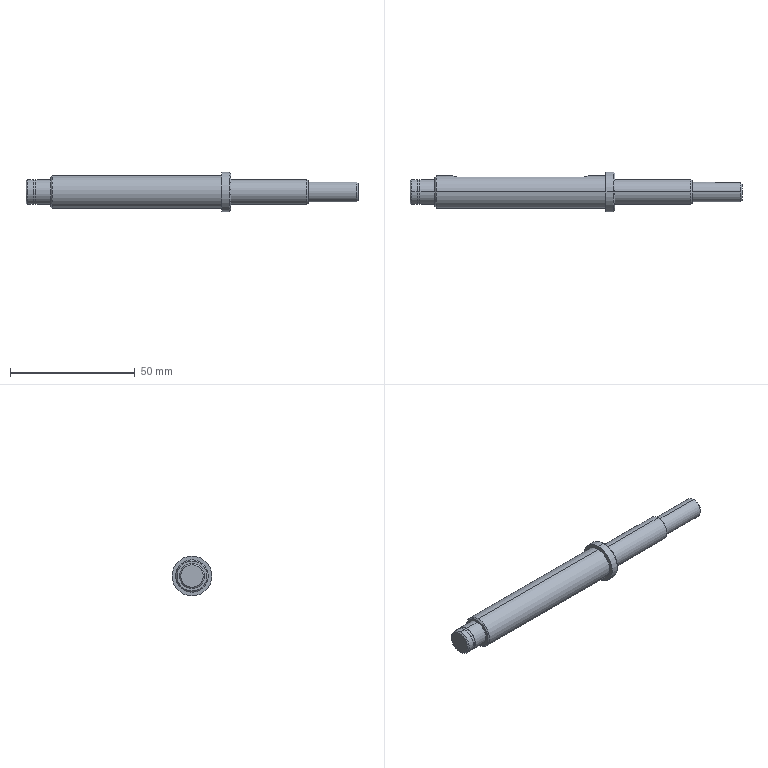Part | SolidWorks | features ICE 2, Chamfer 1, Revolution 1 | 1 solid | 42 faces | box 133 x 16 x 16 mm | volume 13170 mm3 | cylinder 17 | plane 14 | cone 11 | commonest cylinder face diameters 10 x6 5 x2 8 x2 9.6 x2 13 x2 16 x2
STEP:
#1=CARTESIAN_POINT('',(-133.,0.,4.5));
#2=VERTEX_POINT('',#1);
#3=CARTESIAN_POINT('',(-133.,0.,-4.5));
#4=VERTEX_POINT('',#3);
#5=CARTESIAN_POINT('',(-133.,0.,0.));
#6=DIRECTION('',(-1.,0.,0.));
#7=DIRECTION('',(0.,0.,1.));
#8=AXIS2_PLACEMENT_3D('',#5,#6,#7);
#9=CIRCLE('',#8,4.5);
#10=EDGE_CURVE('',#2,#4,#9,.T.);
#11=ORIENTED_EDGE('',*,*,#10,.F.);
#12=CARTESIAN_POINT('',(-132.5,0.,5.));
#13=VERTEX_POINT('',#12);
#14=CARTESIAN_POINT('',(-132.5,0.,5.));
#15=DIRECTION('',(0.7071,0.,0.7071));
#16=VECTOR('',#15,1000.);
#17=LINE('',#14,#16);
#18=EDGE_CURVE('',#2,#13,#17,.T.);
#19=ORIENTED_EDGE('',*,*,#18,.T.);
#20=CARTESIAN_POINT('',(-132.5,0.,-5.));
#21=VERTEX_POINT('',#20);
#22=CARTESIAN_POINT('',(-132.5,0.,0.));
#23=DIRECTION('',(1.,0.,0.));
#24=DIRECTION('',(0.,0.,1.));
#25=AXIS2_PLACEMENT_3D('',#22,#23,#24);
#26=CIRCLE('',#25,5.);
#27=EDGE_CURVE('',#21,#13,#26,.T.);
#28=ORIENTED_EDGE('',*,*,#27,.F.);
#29=CARTESIAN_POINT('',(-132.5,0.,-5.));
#30=DIRECTION('',(0.7071,0.,-0.7071));
#31=VECTOR('',#30,1000.);
#32=LINE('',#29,#31);
#33=EDGE_CURVE('',#4,#21,#32,.T.);
#34=ORIENTED_EDGE('',*,*,#33,.F.);
#35=EDGE_LOOP('',(#11,#19,#28,#34));
#36=FACE_OUTER_BOUND('',#35,.T.);
#37=CARTESIAN_POINT('',(-132.5,0.,0.));
#38=DIRECTION('',(1.,0.,0.));
#39=DIRECTION('',(0.,0.,-1.));
#40=AXIS2_PLACEMENT_3D('',#37,#38,#39);
#41=CONICAL_SURFACE('',#40,5.,0.7854);
#42=ADVANCED_FACE('',(#36),#41,.T.);
#43=CARTESIAN_POINT('',(0.,0.,-3.5));
#44=VERTEX_POINT('',#43);
#45=CARTESIAN_POINT('',(0.,3.162,-1.5));
#46=VERTEX_POINT('',#45);
#47=CARTESIAN_POINT('',(0.,0.,0.));
#48=DIRECTION('',(1.,0.,0.));
#49=DIRECTION('',(0.,0.,-1.));
#50=AXIS2_PLACEMENT_3D('',#47,#48,#49);
#51=CIRCLE('',#50,3.5);
#52=EDGE_CURVE('',#44,#46,#51,.T.);
#53=ORIENTED_EDGE('',*,*,#52,.F.);
#54=CARTESIAN_POINT('',(-0.5,0.,-4.));
#55=VERTEX_POINT('',#54);
#56=CARTESIAN_POINT('',(0.,0.,-3.5));
#57=DIRECTION('',(-0.7071,0.,-0.7071));
#58=VECTOR('',#57,1000.);
#59=LINE('',#56,#58);
#60=EDGE_CURVE('',#44,#55,#59,.T.);
#61=ORIENTED_EDGE('',*,*,#60,.T.);
#62=CARTESIAN_POINT('',(-0.5,3.708,-1.5));
#63=VERTEX_POINT('',#62);
#64=CARTESIAN_POINT('',(-0.5,0.,0.));
#65=DIRECTION('',(-1.,0.,0.));
#66=DIRECTION('',(0.,0.,-1.));
#67=AXIS2_PLACEMENT_3D('',#64,#65,#66);
#68=CIRCLE('',#67,4.);
#69=EDGE_CURVE('',#63,#55,#68,.T.);
#70=ORIENTED_EDGE('',*,*,#69,.F.);
#71=CARTESIAN_POINT('',(0.,3.162,-1.5));
#72=CARTESIAN_POINT('',(-0.1654,3.345,-1.5));
#73=CARTESIAN_POINT('',(-0.3323,3.527,-1.5));
#74=CARTESIAN_POINT('',(-0.5,3.708,-1.5));
#75=B_SPLINE_CURVE_WITH_KNOTS('',3,(#71,#72,#73,#74),.UNSPECIFIED.,.F.,.F.,(4,4),(0.,0.0007402),.UNSPECIFIED.);
#76=EDGE_CURVE('',#46,#63,#75,.T.);
#77=ORIENTED_EDGE('',*,*,#76,.F.);
#78=EDGE_LOOP('',(#53,#61,#70,#77));
#79=FACE_OUTER_BOUND('',#78,.T.);
#80=CARTESIAN_POINT('',(0.,0.,0.));
#81=DIRECTION('',(-1.,0.,0.));
#82=DIRECTION('',(0.,0.,1.));
#83=AXIS2_PLACEMENT_3D('',#80,#81,#82);
#84=CONICAL_SURFACE('',#83,3.5,0.7854);
#85=ADVANCED_FACE('',(#79),#84,.T.);
#86=ORIENTED_EDGE('',*,*,#60,.F.);
#87=CARTESIAN_POINT('',(0.,0.,3.5));
#88=VERTEX_POINT('',#87);
#89=CARTESIAN_POINT('',(0.,0.,0.));
#90=DIRECTION('',(1.,0.,0.));
#91=DIRECTION('',(0.,0.,-1.));
#92=AXIS2_PLACEMENT_3D('',#89,#90,#91);
#93=CIRCLE('',#92,3.5);
#94=EDGE_CURVE('',#88,#44,#93,.T.);
#95=ORIENTED_EDGE('',*,*,#94,.F.);
#96=CARTESIAN_POINT('',(-0.5,0.,4.));
#97=VERTEX_POINT('',#96);
#98=CARTESIAN_POINT('',(0.,0.,3.5));
#99=DIRECTION('',(-0.7071,0.,0.7071));
#100=VECTOR('',#99,1000.);
#101=LINE('',#98,#100);
#102=EDGE_CURVE('',#88,#97,#101,.T.);
#103=ORIENTED_EDGE('',*,*,#102,.T.);
#104=CARTESIAN_POINT('',(-0.5,0.,0.));
#105=DIRECTION('',(-1.,0.,0.));
#106=DIRECTION('',(0.,0.,-1.));
#107=AXIS2_PLACEMENT_3D('',#104,#105,#106);
#108=CIRCLE('',#107,4.);
#109=EDGE_CURVE('',#55,#97,#108,.T.);
#110=ORIENTED_EDGE('',*,*,#109,.F.);
#111=EDGE_LOOP('',(#86,#95,#103,#110));
#112=FACE_OUTER_BOUND('',#111,.T.);
#113=CARTESIAN_POINT('',(0.,0.,0.));
#114=DIRECTION('',(-1.,0.,0.));
#115=DIRECTION('',(0.,0.,1.));
#116=AXIS2_PLACEMENT_3D('',#113,#114,#115);
#117=CONICAL_SURFACE('',#116,3.5,0.7854);
#118=ADVANCED_FACE('',(#112),#117,.T.);
#119=CARTESIAN_POINT('',(-20.,0.,-4.5));
#120=VERTEX_POINT('',#119);
#121=CARTESIAN_POINT('',(-20.,0.,4.5));
#122=VERTEX_POINT('',#121);
#123=CARTESIAN_POINT('',(-20.,0.,0.));
#124=DIRECTION('',(1.,0.,0.));
#125=DIRECTION('',(0.,0.,-1.));
#126=AXIS2_PLACEMENT_3D('',#123,#124,#125);
#127=CIRCLE('',#126,4.5);
#128=EDGE_CURVE('',#120,#122,#127,.T.);
#129=ORIENTED_EDGE('',*,*,#128,.F.);
#130=CARTESIAN_POINT('',(-20.5,0.,-5.));
#131=VERTEX_POINT('',#130);
#132=CARTESIAN_POINT('',(-20.,0.,-4.5));
#133=DIRECTION('',(-0.7071,0.,-0.7071));
#134=VECTOR('',#133,1000.);
#135=LINE('',#132,#134);
#136=EDGE_CURVE('',#120,#131,#135,.T.);
#137=ORIENTED_EDGE('',*,*,#136,.T.);
#138=CARTESIAN_POINT('',(-20.5,0.,5.));
#139=VERTEX_POINT('',#138);
#140=CARTESIAN_POINT('',(-20.5,0.,0.));
#141=DIRECTION('',(-1.,0.,0.));
#142=DIRECTION('',(0.,0.,-1.));
#143=AXIS2_PLACEMENT_3D('',#140,#141,#142);
#144=CIRCLE('',#143,5.);
#145=EDGE_CURVE('',#139,#131,#144,.T.);
#146=ORIENTED_EDGE('',*,*,#145,.F.);
#147=CARTESIAN_POINT('',(-20.,0.,4.5));
#148=DIRECTION('',(-0.7071,0.,0.7071));
#149=VECTOR('',#148,1000.);
#150=LINE('',#147,#149);
#151=EDGE_CURVE('',#122,#139,#150,.T.);
#152=ORIENTED_EDGE('',*,*,#151,.F.);
#153=EDGE_LOOP('',(#129,#137,#146,#152));
#154=FACE_OUTER_BOUND('',#153,.T.);
#155=CARTESIAN_POINT('',(-20.,0.,0.));
#156=DIRECTION('',(-1.,0.,0.));
#157=DIRECTION('',(0.,0.,1.));
#158=AXIS2_PLACEMENT_3D('',#155,#156,#157);
#159=CONICAL_SURFACE('',#158,4.5,0.7854);
#160=ADVANCED_FACE('',(#154),#159,.T.);
#161=CARTESIAN_POINT('',(-123.,0.,6.));
#162=VERTEX_POINT('',#161);
#163=CARTESIAN_POINT('',(-123.,0.,-6.));
#164=VERTEX_POINT('',#163);
#165=CARTESIAN_POINT('',(-123.,0.,0.));
#166=DIRECTION('',(-1.,0.,0.));
#167=DIRECTION('',(0.,0.,1.));
#168=AXIS2_PLACEMENT_3D('',#165,#166,#167);
#169=CIRCLE('',#168,6.);
#170=EDGE_CURVE('',#162,#164,#169,.T.);
#171=ORIENTED_EDGE('',*,*,#170,.F.);
#172=CARTESIAN_POINT('',(-122.5,0.,6.5));
#173=VERTEX_POINT('',#172);
#174=CARTESIAN_POINT('',(-122.5,0.,6.5));
#175=DIRECTION('',(0.7071,0.,0.7071));
#176=VECTOR('',#175,1000.);
#177=LINE('',#174,#176);
#178=EDGE_CURVE('',#162,#173,#177,.T.);
#179=ORIENTED_EDGE('',*,*,#178,.T.);
#180=CARTESIAN_POINT('',(-122.5,0.,-6.5));
#181=VERTEX_POINT('',#180);
#182=CARTESIAN_POINT('',(-122.5,0.,0.));
#183=DIRECTION('',(1.,0.,0.));
#184=DIRECTION('',(0.,0.,1.));
#185=AXIS2_PLACEMENT_3D('',#182,#183,#184);
#186=CIRCLE('',#185,6.5);
#187=EDGE_CURVE('',#181,#173,#186,.T.);
#188=ORIENTED_EDGE('',*,*,#187,.F.);
#189=CARTESIAN_POINT('',(-122.5,0.,-6.5));
#190=DIRECTION('',(0.7071,0.,-0.7071));
#191=VECTOR('',#190,1000.);
#192=LINE('',#189,#191);
#193=EDGE_CURVE('',#164,#181,#192,.T.);
#194=ORIENTED_EDGE('',*,*,#193,.F.);
#195=EDGE_LOOP('',(#171,#179,#188,#194));
#196=FACE_OUTER_BOUND('',#195,.T.);
#197=CARTESIAN_POINT('',(-122.5,0.,0.));
#198=DIRECTION('',(1.,0.,0.));
#199=DIRECTION('',(0.,0.,-1.));
#200=AXIS2_PLACEMENT_3D('',#197,#198,#199);
#201=CONICAL_SURFACE('',#200,6.5,0.7854);
#202=ADVANCED_FACE('',(#196),#201,.T.);
#203=CARTESIAN_POINT('',(-51.,0.,-7.5));
#204=VERTEX_POINT('',#203);
#205=CARTESIAN_POINT('',(-51.,0.,7.5));
#206=VERTEX_POINT('',#205);
#207=CARTESIAN_POINT('',(-51.,0.,0.));
#208=DIRECTION('',(1.,0.,0.));
#209=DIRECTION('',(0.,0.,-1.));
#210=AXIS2_PLACEMENT_3D('',#207,#208,#209);
#211=CIRCLE('',#210,7.5);
#212=EDGE_CURVE('',#204,#206,#211,.T.);
#213=ORIENTED_EDGE('',*,*,#212,.F.);
#214=CARTESIAN_POINT('',(-51.5,0.,-8.));
#215=VERTEX_POINT('',#214);
#216=CARTESIAN_POINT('',(-51.,0.,-7.5));
#217=DIRECTION('',(-0.7071,0.,-0.7071));
#218=VECTOR('',#217,1000.);
#219=LINE('',#216,#218);
#220=EDGE_CURVE('',#204,#215,#219,.T.);
#221=ORIENTED_EDGE('',*,*,#220,.T.);
#222=CARTESIAN_POINT('',(-51.5,0.,8.));
#223=VERTEX_POINT('',#222);
#224=CARTESIAN_POINT('',(-51.5,0.,0.));
#225=DIRECTION('',(-1.,0.,0.));
#226=DIRECTION('',(0.,0.,-1.));
#227=AXIS2_PLACEMENT_3D('',#224,#225,#226);
#228=CIRCLE('',#227,8.);
#229=EDGE_CURVE('',#223,#215,#228,.T.);
#230=ORIENTED_EDGE('',*,*,#229,.F.);
#231=CARTESIAN_POINT('',(-51.,0.,7.5));
#232=DIRECTION('',(-0.7071,0.,0.7071));
#233=VECTOR('',#232,1000.);
#234=LINE('',#231,#233);
#235=EDGE_CURVE('',#206,#223,#234,.T.);
#236=ORIENTED_EDGE('',*,*,#235,.F.);
#237=EDGE_LOOP('',(#213,#221,#230,#236));
#238=FACE_OUTER_BOUND('',#237,.T.);
#239=CARTESIAN_POINT('',(-51.,0.,0.));
#240=DIRECTION('',(-1.,0.,0.));
#241=DIRECTION('',(0.,0.,1.));
#242=AXIS2_PLACEMENT_3D('',#239,#240,#241);
#243=CONICAL_SURFACE('',#242,7.5,0.7854);
#244=ADVANCED_FACE('',(#238),#243,.T.);
#245=CARTESIAN_POINT('',(-20.,0.,-4.));
#246=VERTEX_POINT('',#245);
#247=CARTESIAN_POINT('',(-20.,0.,4.));
#248=VERTEX_POINT('',#247);
#249=CARTESIAN_POINT('',(-20.,0.,0.));
#250=DIRECTION('',(1.,0.,0.));
#251=DIRECTION('',(0.,0.,-1.));
#252=AXIS2_PLACEMENT_3D('',#249,#250,#251);
#253=CIRCLE('',#252,4.);
#254=EDGE_CURVE('',#246,#248,#253,.T.);
#255=ORIENTED_EDGE('',*,*,#254,.T.);
#256=CARTESIAN_POINT('',(0.,0.,4.));
#257=DIRECTION('',(1.,0.,0.));
#258=VECTOR('',#257,1000.);
#259=LINE('',#256,#258);
#260=EDGE_CURVE('',#248,#97,#259,.T.);
#261=ORIENTED_EDGE('',*,*,#260,.T.);
#262=CARTESIAN_POINT('',(-0.5,3.708,1.5));
#263=VERTEX_POINT('',#262);
#264=CARTESIAN_POINT('',(-0.5,0.,0.));
#265=DIRECTION('',(-1.,0.,0.));
#266=DIRECTION('',(0.,0.,-1.));
#267=AXIS2_PLACEMENT_3D('',#264,#265,#266);
#268=CIRCLE('',#267,4.);
#269=EDGE_CURVE('',#97,#263,#268,.T.);
#270=ORIENTED_EDGE('',*,*,#269,.T.);
#271=CARTESIAN_POINT('',(-10.,3.708,1.5));
#272=VERTEX_POINT('',#271);
#273=CARTESIAN_POINT('',(0.,3.708,1.5));
#274=DIRECTION('',(1.,0.,0.));
#275=VECTOR('',#274,1000.);
#276=LINE('',#273,#275);
#277=EDGE_CURVE('',#272,#263,#276,.T.);
#278=ORIENTED_EDGE('',*,*,#277,.F.);
#279=CARTESIAN_POINT('',(-10.,3.708,-1.5));
#280=VERTEX_POINT('',#279);
#281=CARTESIAN_POINT('',(-10.,3.708,-1.5));
#282=CARTESIAN_POINT('',(-10.1,3.708,-1.5));
#283=CARTESIAN_POINT('',(-10.198,3.712,-1.49));
#284=CARTESIAN_POINT('',(-10.391,3.727,-1.451));
#285=CARTESIAN_POINT('',(-10.487,3.739,-1.422));
#286=CARTESIAN_POINT('',(-10.758,3.781,-1.309));
#287=CARTESIAN_POINT('',(-10.923,3.819,-1.198));
#288=CARTESIAN_POINT('',(-11.197,3.894,-0.924));
#289=CARTESIAN_POINT('',(-11.309,3.932,-0.7582));
#290=CARTESIAN_POINT('',(-11.422,3.971,-0.488));
#291=CARTESIAN_POINT('',(-11.451,3.982,-0.3926));
#292=CARTESIAN_POINT('',(-11.49,3.996,-0.1986));
#293=CARTESIAN_POINT('',(-11.5,4.,-0.1006));
#294=CARTESIAN_POINT('',(-11.5,4.,0.09712));
#295=CARTESIAN_POINT('',(-11.49,3.996,0.1975));
#296=CARTESIAN_POINT('',(-11.452,3.982,0.3907));
#297=CARTESIAN_POINT('',(-11.423,3.972,0.4847));
#298=CARTESIAN_POINT('',(-11.309,3.932,0.759));
#299=CARTESIAN_POINT('',(-11.198,3.895,0.9229));
#300=CARTESIAN_POINT('',(-10.992,3.838,1.129));
#301=CARTESIAN_POINT('',(-10.917,3.819,1.191));
#302=CARTESIAN_POINT('',(-10.756,3.783,1.299));
#303=CARTESIAN_POINT('',(-10.668,3.767,1.347));
#304=CARTESIAN_POINT('',(-10.398,3.725,1.459));
#305=CARTESIAN_POINT('',(-10.2,3.708,1.5));
#306=CARTESIAN_POINT('',(-10.,3.708,1.5));
#307=B_SPLINE_CURVE_WITH_KNOTS('',3,(#281,#282,#283,#284,#285,#286,#287,#288,#289,#290,#291,#292,#293,#294,#295,#296,#297,#298,#299,#300,#301,#302,#303,#304,#305,#306),.UNSPECIFIED.,.F.,.F.,(4,2,2,2,2,2,2,2,2,2,2,2,4),(0.,0.0002957,0.0005914,0.001183,0.001774,0.00207,0.002366,0.002661,0.002957,0.003548,0.003844,0.00414,0.004731),.UNSPECIFIED.);
#308=EDGE_CURVE('',#280,#272,#307,.T.);
#309=ORIENTED_EDGE('',*,*,#308,.F.);
#310=CARTESIAN_POINT('',(0.,3.708,-1.5));
#311=DIRECTION('',(-1.,0.,0.));
#312=VECTOR('',#311,1000.);
#313=LINE('',#310,#312);
#314=EDGE_CURVE('',#63,#280,#313,.T.);
#315=ORIENTED_EDGE('',*,*,#314,.F.);
#316=ORIENTED_EDGE('',*,*,#69,.T.);
#317=CARTESIAN_POINT('',(0.,0.,-4.));
#318=DIRECTION('',(1.,0.,0.));
#319=VECTOR('',#318,1000.);
#320=LINE('',#317,#319);
#321=EDGE_CURVE('',#246,#55,#320,.T.);
#322=ORIENTED_EDGE('',*,*,#321,.F.);
#323=EDGE_LOOP('',(#255,#261,#270,#278,#309,#315,#316,#322));
#324=FACE_OUTER_BOUND('',#323,.T.);
#325=CARTESIAN_POINT('',(0.,0.,0.));
#326=DIRECTION('',(1.,0.,0.));
#327=DIRECTION('',(0.,0.,-1.));
#328=AXIS2_PLACEMENT_3D('',#325,#326,#327);
#329=CYLINDRICAL_SURFACE('',#328,4.);
#330=ADVANCED_FACE('',(#324),#329,.T.);
#331=CARTESIAN_POINT('',(-51.,0.,-5.));
#332=VERTEX_POINT('',#331);
#333=CARTESIAN_POINT('',(-51.,0.,5.));
#334=VERTEX_POINT('',#333);
#335=CARTESIAN_POINT('',(-51.,0.,0.));
#336=DIRECTION('',(1.,0.,0.));
#337=DIRECTION('',(0.,0.,-1.));
#338=AXIS2_PLACEMENT_3D('',#335,#336,#337);
#339=CIRCLE('',#338,5.);
#340=EDGE_CURVE('',#332,#334,#339,.T.);
#341=ORIENTED_EDGE('',*,*,#340,.T.);
#342=CARTESIAN_POINT('',(0.,0.,5.));
#343=DIRECTION('',(1.,0.,0.));
#344=VECTOR('',#343,1000.);
#345=LINE('',#342,#344);
#346=EDGE_CURVE('',#334,#139,#345,.T.);
#347=ORIENTED_EDGE('',*,*,#346,.T.);
#348=ORIENTED_EDGE('',*,*,#145,.T.);
#349=CARTESIAN_POINT('',(0.,0.,-5.));
#350=DIRECTION('',(1.,0.,0.));
#351=VECTOR('',#350,1000.);
#352=LINE('',#349,#351);
#353=EDGE_CURVE('',#332,#131,#352,.T.);
#354=ORIENTED_EDGE('',*,*,#353,.F.);
#355=EDGE_LOOP('',(#341,#347,#348,#354));
#356=FACE_OUTER_BOUND('',#355,.T.);
#357=CARTESIAN_POINT('',(0.,0.,0.));
#358=DIRECTION('',(1.,0.,0.));
#359=DIRECTION('',(0.,0.,-1.));
#360=AXIS2_PLACEMENT_3D('',#357,#358,#359);
#361=CYLINDRICAL_SURFACE('',#360,5.);
#362=ADVANCED_FACE('',(#356),#361,.T.);
#363=CARTESIAN_POINT('',(-54.5,0.,-8.));
#364=VERTEX_POINT('',#363);
#365=CARTESIAN_POINT('',(-54.5,0.,8.));
#366=VERTEX_POINT('',#365);
#367=CARTESIAN_POINT('',(-54.5,0.,0.));
#368=DIRECTION('',(1.,0.,0.));
#369=DIRECTION('',(0.,0.,-1.));
#370=AXIS2_PLACEMENT_3D('',#367,#368,#369);
#371=CIRCLE('',#370,8.);
#372=EDGE_CURVE('',#364,#366,#371,.T.);
#373=ORIENTED_EDGE('',*,*,#372,.T.);
#374=CARTESIAN_POINT('',(0.,0.,8.));
#375=DIRECTION('',(1.,0.,0.));
#376=VECTOR('',#375,1000.);
#377=LINE('',#374,#376);
#378=EDGE_CURVE('',#366,#223,#377,.T.);
#379=ORIENTED_EDGE('',*,*,#378,.T.);
#380=ORIENTED_EDGE('',*,*,#229,.T.);
#381=CARTESIAN_POINT('',(0.,0.,-8.));
#382=DIRECTION('',(1.,0.,0.));
#383=VECTOR('',#382,1000.);
#384=LINE('',#381,#383);
#385=EDGE_CURVE('',#364,#215,#384,.T.);
#386=ORIENTED_EDGE('',*,*,#385,.F.);
#387=EDGE_LOOP('',(#373,#379,#380,#386));
#388=FACE_OUTER_BOUND('',#387,.T.);
#389=CARTESIAN_POINT('',(0.,0.,0.));
#390=DIRECTION('',(1.,0.,0.));
#391=DIRECTION('',(0.,0.,-1.));
#392=AXIS2_PLACEMENT_3D('',#389,#390,#391);
#393=CYLINDRICAL_SURFACE('',#392,8.);
#394=ADVANCED_FACE('',(#388),#393,.T.);
#395=CARTESIAN_POINT('',(-63.75,6.,2.5));
#396=VERTEX_POINT('',#395);
#397=CARTESIAN_POINT('',(-63.75,6.,-2.5));
#398=VERTEX_POINT('',#397);
#399=CARTESIAN_POINT('',(-63.75,6.,2.5));
#400=CARTESIAN_POINT('',(-63.583,6.,2.5));
#401=CARTESIAN_POINT('',(-63.419,6.007,2.483));
#402=CARTESIAN_POINT('',(-63.098,6.033,2.419));
#403=CARTESIAN_POINT('',(-62.938,6.053,2.37));
#404=CARTESIAN_POINT('',(-62.637,6.101,2.244));
#405=CARTESIAN_POINT('',(-62.494,6.129,2.168));
#406=CARTESIAN_POINT('',(-62.223,6.19,1.986));
#407=CARTESIAN_POINT('',(-62.097,6.223,1.882));
#408=CARTESIAN_POINT('',(-61.754,6.319,1.54));
#409=CARTESIAN_POINT('',(-61.569,6.383,1.264));
#410=CARTESIAN_POINT('',(-61.381,6.451,0.8138));
#411=CARTESIAN_POINT('',(-61.332,6.469,0.6546));
#412=CARTESIAN_POINT('',(-61.267,6.494,0.3312));
#413=CARTESIAN_POINT('',(-61.25,6.5,0.1679));
#414=CARTESIAN_POINT('',(-61.25,6.5,-0.1619));
#415=CARTESIAN_POINT('',(-61.266,6.494,-0.3292));
#416=CARTESIAN_POINT('',(-61.331,6.469,-0.6513));
#417=CARTESIAN_POINT('',(-61.378,6.451,-0.8081));
#418=CARTESIAN_POINT('',(-61.505,6.406,-1.113));
#419=CARTESIAN_POINT('',(-61.583,6.379,-1.256));
#420=CARTESIAN_POINT('',(-61.763,6.32,-1.526));
#421=CARTESIAN_POINT('',(-61.868,6.287,-1.653));
#422=CARTESIAN_POINT('',(-62.097,6.223,-1.882));
#423=CARTESIAN_POINT('',(-62.221,6.19,-1.985));
#424=CARTESIAN_POINT('',(-62.491,6.129,-2.166));
#425=CARTESIAN_POINT('',(-62.636,6.101,-2.244));
#426=CARTESIAN_POINT('',(-63.086,6.029,-2.432));
#427=CARTESIAN_POINT('',(-63.416,6.,-2.5));
#428=CARTESIAN_POINT('',(-63.75,6.,-2.5));
#429=B_SPLINE_CURVE_WITH_KNOTS('',3,(#399,#400,#401,#402,#403,#404,#405,#406,#407,#408,#409,#410,#411,#412,#413,#414,#415,#416,#417,#418,#419,#420,#421,#422,#423,#424,#425,#426,#427,#428),.UNSPECIFIED.,.F.,.F.,(4,2,2,2,2,2,2,2,2,2,2,2,2,2,4),(0.,0.0004931,0.0009861,0.001479,0.001972,0.002958,0.003452,0.003945,0.004438,0.004931,0.005424,0.005917,0.00641,0.006903,0.007889),.UNSPECIFIED.);
#430=EDGE_CURVE('',#396,#398,#429,.T.);
#431=ORIENTED_EDGE('',*,*,#430,.F.);
#432=CARTESIAN_POINT('',(-113.75,6.,2.5));
#433=VERTEX_POINT('',#432);
#434=CARTESIAN_POINT('',(0.,6.,2.5));
#435=DIRECTION('',(1.,0.,0.));
#436=VECTOR('',#435,1000.);
#437=LINE('',#434,#436);
#438=EDGE_CURVE('',#433,#396,#437,.T.);
#439=ORIENTED_EDGE('',*,*,#438,.F.);
#440=CARTESIAN_POINT('',(-113.75,6.,-2.5));
#441=VERTEX_POINT('',#440);
#442=CARTESIAN_POINT('',(-113.75,6.,-2.5));
#443=CARTESIAN_POINT('',(-113.917,6.,-2.5));
#444=CARTESIAN_POINT('',(-114.081,6.007,-2.483));
#445=CARTESIAN_POINT('',(-114.402,6.033,-2.419));
#446=CARTESIAN_POINT('',(-114.562,6.053,-2.37));
#447=CARTESIAN_POINT('',(-114.863,6.101,-2.244));
#448=CARTESIAN_POINT('',(-115.006,6.129,-2.168));
#449=CARTESIAN_POINT('',(-115.277,6.19,-1.986));
#450=CARTESIAN_POINT('',(-115.403,6.223,-1.882));
#451=CARTESIAN_POINT('',(-115.746,6.319,-1.54));
#452=CARTESIAN_POINT('',(-115.931,6.383,-1.264));
#453=CARTESIAN_POINT('',(-116.119,6.451,-0.8138));
#454=CARTESIAN_POINT('',(-116.168,6.469,-0.6546));
#455=CARTESIAN_POINT('',(-116.233,6.494,-0.3312));
#456=CARTESIAN_POINT('',(-116.25,6.5,-0.1679));
#457=CARTESIAN_POINT('',(-116.25,6.5,0.1619));
#458=CARTESIAN_POINT('',(-116.234,6.494,0.3292));
#459=CARTESIAN_POINT('',(-116.169,6.469,0.6513));
#460=CARTESIAN_POINT('',(-116.122,6.451,0.8081));
#461=CARTESIAN_POINT('',(-115.995,6.406,1.113));
#462=CARTESIAN_POINT('',(-115.917,6.379,1.256));
#463=CARTESIAN_POINT('',(-115.737,6.32,1.526));
#464=CARTESIAN_POINT('',(-115.632,6.287,1.653));
#465=CARTESIAN_POINT('',(-115.403,6.223,1.882));
#466=CARTESIAN_POINT('',(-115.279,6.19,1.985));
#467=CARTESIAN_POINT('',(-115.009,6.129,2.166));
#468=CARTESIAN_POINT('',(-114.864,6.101,2.244));
#469=CARTESIAN_POINT('',(-114.414,6.029,2.432));
#470=CARTESIAN_POINT('',(-114.084,6.,2.5));
#471=CARTESIAN_POINT('',(-113.75,6.,2.5));
#472=B_SPLINE_CURVE_WITH_KNOTS('',3,(#442,#443,#444,#445,#446,#447,#448,#449,#450,#451,#452,#453,#454,#455,#456,#457,#458,#459,#460,#461,#462,#463,#464,#465,#466,#467,#468,#469,#470,#471),.UNSPECIFIED.,.F.,.F.,(4,2,2,2,2,2,2,2,2,2,2,2,2,2,4),(0.,0.0004931,0.0009861,0.001479,0.001972,0.002958,0.003452,0.003945,0.004438,0.004931,0.005424,0.005917,0.00641,0.006903,0.007889),.UNSPECIFIED.);
#473=EDGE_CURVE('',#441,#433,#472,.T.);
#474=ORIENTED_EDGE('',*,*,#473,.F.);
#475=CARTESIAN_POINT('',(0.,6.,-2.5));
#476=DIRECTION('',(-1.,0.,0.));
#477=VECTOR('',#476,1000.);
#478=LINE('',#475,#477);
#479=EDGE_CURVE('',#398,#441,#478,.T.);
#480=ORIENTED_EDGE('',*,*,#479,.F.);
#481=EDGE_LOOP('',(#431,#439,#474,#480));
#482=FACE_BOUND('',#481,.T.);
#483=ORIENTED_EDGE('',*,*,#187,.T.);
#484=CARTESIAN_POINT('',(-54.5,0.,6.5));
#485=VERTEX_POINT('',#484);
#486=CARTESIAN_POINT('',(0.,0.,6.5));
#487=DIRECTION('',(1.,0.,0.));
#488=VECTOR('',#487,1000.);
#489=LINE('',#486,#488);
#490=EDGE_CURVE('',#173,#485,#489,.T.);
#491=ORIENTED_EDGE('',*,*,#490,.T.);
#492=CARTESIAN_POINT('',(-54.5,0.,-6.5));
#493=VERTEX_POINT('',#492);
#494=CARTESIAN_POINT('',(-54.5,0.,0.));
#495=DIRECTION('',(1.,0.,0.));
#496=DIRECTION('',(0.,0.,-1.));
#497=AXIS2_PLACEMENT_3D('',#494,#495,#496);
#498=CIRCLE('',#497,6.5);
#499=EDGE_CURVE('',#493,#485,#498,.T.);
#500=ORIENTED_EDGE('',*,*,#499,.F.);
#501=CARTESIAN_POINT('',(0.,0.,-6.5));
#502=DIRECTION('',(1.,0.,0.));
#503=VECTOR('',#502,1000.);
#504=LINE('',#501,#503);
#505=EDGE_CURVE('',#181,#493,#504,.T.);
#506=ORIENTED_EDGE('',*,*,#505,.F.);
#507=EDGE_LOOP('',(#483,#491,#500,#506));
#508=FACE_OUTER_BOUND('',#507,.T.);
#509=CARTESIAN_POINT('',(0.,0.,0.));
#510=DIRECTION('',(1.,0.,0.));
#511=DIRECTION('',(0.,0.,-1.));
#512=AXIS2_PLACEMENT_3D('',#509,#510,#511);
#513=CYLINDRICAL_SURFACE('',#512,6.5);
#514=ADVANCED_FACE('',(#482,#508),#513,.T.);
#515=CARTESIAN_POINT('',(-129.,0.,-5.));
#516=VERTEX_POINT('',#515);
#517=CARTESIAN_POINT('',(-129.,0.,5.));
#518=VERTEX_POINT('',#517);
#519=CARTESIAN_POINT('',(-129.,0.,0.));
#520=DIRECTION('',(1.,0.,0.));
#521=DIRECTION('',(0.,0.,-1.));
#522=AXIS2_PLACEMENT_3D('',#519,#520,#521);
#523=CIRCLE('',#522,5.);
#524=EDGE_CURVE('',#516,#518,#523,.T.);
#525=ORIENTED_EDGE('',*,*,#524,.T.);
#526=CARTESIAN_POINT('',(-123.,0.,5.));
#527=VERTEX_POINT('',#526);
#528=CARTESIAN_POINT('',(0.,0.,5.));
#529=DIRECTION('',(1.,0.,0.));
#530=VECTOR('',#529,1000.);
#531=LINE('',#528,#530);
#532=EDGE_CURVE('',#518,#527,#531,.T.);
#533=ORIENTED_EDGE('',*,*,#532,.T.);
#534=CARTESIAN_POINT('',(-123.,0.,-5.));
#535=VERTEX_POINT('',#534);
#536=CARTESIAN_POINT('',(-123.,0.,0.));
#537=DIRECTION('',(1.,0.,0.));
#538=DIRECTION('',(0.,0.,-1.));
#539=AXIS2_PLACEMENT_3D('',#536,#537,#538);
#540=CIRCLE('',#539,5.);
#541=EDGE_CURVE('',#535,#527,#540,.T.);
#542=ORIENTED_EDGE('',*,*,#541,.F.);
#543=CARTESIAN_POINT('',(0.,0.,-5.));
#544=DIRECTION('',(1.,0.,0.));
#545=VECTOR('',#544,1000.);
#546=LINE('',#543,#545);
#547=EDGE_CURVE('',#516,#535,#546,.T.);
#548=ORIENTED_EDGE('',*,*,#547,.F.);
#549=EDGE_LOOP('',(#525,#533,#542,#548));
#550=FACE_OUTER_BOUND('',#549,.T.);
#551=CARTESIAN_POINT('',(0.,0.,0.));
#552=DIRECTION('',(1.,0.,0.));
#553=DIRECTION('',(0.,0.,-1.));
#554=AXIS2_PLACEMENT_3D('',#551,#552,#553);
#555=CYLINDRICAL_SURFACE('',#554,5.);
#556=ADVANCED_FACE('',(#550),#555,.T.);
#557=CARTESIAN_POINT('',(-130.1,0.,-4.8));
#558=VERTEX_POINT('',#557);
#559=CARTESIAN_POINT('',(-130.1,0.,4.8));
#560=VERTEX_POINT('',#559);
#561=CARTESIAN_POINT('',(-130.1,0.,0.));
#562=DIRECTION('',(1.,0.,0.));
#563=DIRECTION('',(0.,0.,-1.));
#564=AXIS2_PLACEMENT_3D('',#561,#562,#563);
#565=CIRCLE('',#564,4.8);
#566=EDGE_CURVE('',#558,#560,#565,.T.);
#567=ORIENTED_EDGE('',*,*,#566,.T.);
#568=CARTESIAN_POINT('',(-129.,0.,4.8));
#569=VERTEX_POINT('',#568);
#570=CARTESIAN_POINT('',(0.,0.,4.8));
#571=DIRECTION('',(1.,0.,0.));
#572=VECTOR('',#571,1000.);
#573=LINE('',#570,#572);
#574=EDGE_CURVE('',#560,#569,#573,.T.);
#575=ORIENTED_EDGE('',*,*,#574,.T.);
#576=CARTESIAN_POINT('',(-129.,0.,-4.8));
#577=VERTEX_POINT('',#576);
#578=CARTESIAN_POINT('',(-129.,0.,0.));
#579=DIRECTION('',(1.,0.,0.));
#580=DIRECTION('',(0.,0.,-1.));
#581=AXIS2_PLACEMENT_3D('',#578,#579,#580);
#582=CIRCLE('',#581,4.8);
#583=EDGE_CURVE('',#577,#569,#582,.T.);
#584=ORIENTED_EDGE('',*,*,#583,.F.);
#585=CARTESIAN_POINT('',(0.,0.,-4.8));
#586=DIRECTION('',(1.,0.,0.));
#587=VECTOR('',#586,1000.);
#588=LINE('',#585,#587);
#589=EDGE_CURVE('',#558,#577,#588,.T.);
#590=ORIENTED_EDGE('',*,*,#589,.F.);
#591=EDGE_LOOP('',(#567,#575,#584,#590));
#592=FACE_OUTER_BOUND('',#591,.T.);
#593=CARTESIAN_POINT('',(0.,0.,0.));
#594=DIRECTION('',(1.,0.,0.));
#595=DIRECTION('',(0.,0.,-1.));
#596=AXIS2_PLACEMENT_3D('',#593,#594,#595);
#597=CYLINDRICAL_SURFACE('',#596,4.8);
#598=ADVANCED_FACE('',(#592),#597,.T.);
#599=ORIENTED_EDGE('',*,*,#27,.T.);
#600=CARTESIAN_POINT('',(-130.1,0.,5.));
#601=VERTEX_POINT('',#600);
#602=CARTESIAN_POINT('',(0.,0.,5.));
#603=DIRECTION('',(1.,0.,0.));
#604=VECTOR('',#603,1000.);
#605=LINE('',#602,#604);
#606=EDGE_CURVE('',#13,#601,#605,.T.);
#607=ORIENTED_EDGE('',*,*,#606,.T.);
#608=CARTESIAN_POINT('',(-130.1,0.,-5.));
#609=VERTEX_POINT('',#608);
#610=CARTESIAN_POINT('',(-130.1,0.,0.));
#611=DIRECTION('',(1.,0.,0.));
#612=DIRECTION('',(0.,0.,-1.));
#613=AXIS2_PLACEMENT_3D('',#610,#611,#612);
#614=CIRCLE('',#613,5.);
#615=EDGE_CURVE('',#609,#601,#614,.T.);
#616=ORIENTED_EDGE('',*,*,#615,.F.);
#617=CARTESIAN_POINT('',(0.,0.,-5.));
#618=DIRECTION('',(1.,0.,0.));
#619=VECTOR('',#618,1000.);
#620=LINE('',#617,#619);
#621=EDGE_CURVE('',#21,#609,#620,.T.);
#622=ORIENTED_EDGE('',*,*,#621,.F.);
#623=EDGE_LOOP('',(#599,#607,#616,#622));
#624=FACE_OUTER_BOUND('',#623,.T.);
#625=CARTESIAN_POINT('',(0.,0.,0.));
#626=DIRECTION('',(1.,0.,0.));
#627=DIRECTION('',(0.,0.,-1.));
#628=AXIS2_PLACEMENT_3D('',#625,#626,#627);
#629=CYLINDRICAL_SURFACE('',#628,5.);
#630=ADVANCED_FACE('',(#624),#629,.T.);
#631=CARTESIAN_POINT('',(-133.,0.,0.));
#632=DIRECTION('',(-1.,0.,0.));
#633=DIRECTION('',(0.,0.,1.));
#634=AXIS2_PLACEMENT_3D('',#631,#632,#633);
#635=CIRCLE('',#634,4.5);
#636=EDGE_CURVE('',#4,#2,#635,.T.);
#637=ORIENTED_EDGE('',*,*,#636,.T.);
#638=ORIENTED_EDGE('',*,*,#10,.T.);
#639=EDGE_LOOP('',(#637,#638));
#640=FACE_OUTER_BOUND('',#639,.T.);
#641=CARTESIAN_POINT('',(-133.,5.,0.));
#642=DIRECTION('',(-1.,0.,0.));
#643=DIRECTION('',(0.,0.,1.));
#644=AXIS2_PLACEMENT_3D('',#641,#642,#643);
#645=PLANE('',#644);
#646=ADVANCED_FACE('',(#640),#645,.T.);
#647=ORIENTED_EDGE('',*,*,#606,.F.);
#648=CARTESIAN_POINT('',(-132.5,0.,0.));
#649=DIRECTION('',(1.,0.,0.));
#650=DIRECTION('',(0.,0.,1.));
#651=AXIS2_PLACEMENT_3D('',#648,#649,#650);
#652=CIRCLE('',#651,5.);
#653=EDGE_CURVE('',#13,#21,#652,.T.);
#654=ORIENTED_EDGE('',*,*,#653,.T.);
#655=ORIENTED_EDGE('',*,*,#621,.T.);
#656=CARTESIAN_POINT('',(-130.1,0.,0.));
#657=DIRECTION('',(1.,0.,0.));
#658=DIRECTION('',(0.,0.,-1.));
#659=AXIS2_PLACEMENT_3D('',#656,#657,#658);
#660=CIRCLE('',#659,5.);
#661=EDGE_CURVE('',#601,#609,#660,.T.);
#662=ORIENTED_EDGE('',*,*,#661,.F.);
#663=EDGE_LOOP('',(#647,#654,#655,#662));
#664=FACE_OUTER_BOUND('',#663,.T.);
#665=CARTESIAN_POINT('',(0.,0.,0.));
#666=DIRECTION('',(1.,0.,0.));
#667=DIRECTION('',(0.,0.,-1.));
#668=AXIS2_PLACEMENT_3D('',#665,#666,#667);
#669=CYLINDRICAL_SURFACE('',#668,5.);
#670=ADVANCED_FACE('',(#664),#669,.T.);
#671=ORIENTED_EDGE('',*,*,#615,.T.);
#672=ORIENTED_EDGE('',*,*,#661,.T.);
#673=EDGE_LOOP('',(#671,#672));
#674=FACE_OUTER_BOUND('',#673,.T.);
#675=ORIENTED_EDGE('',*,*,#566,.F.);
#676=CARTESIAN_POINT('',(-130.1,0.,0.));
#677=DIRECTION('',(1.,0.,0.));
#678=DIRECTION('',(0.,0.,-1.));
#679=AXIS2_PLACEMENT_3D('',#676,#677,#678);
#680=CIRCLE('',#679,4.8);
#681=EDGE_CURVE('',#560,#558,#680,.T.);
#682=ORIENTED_EDGE('',*,*,#681,.F.);
#683=EDGE_LOOP('',(#675,#682));
#684=FACE_BOUND('',#683,.T.);
#685=CARTESIAN_POINT('',(-130.1,4.8,0.));
#686=DIRECTION('',(1.,0.,0.));
#687=DIRECTION('',(0.,0.,-1.));
#688=AXIS2_PLACEMENT_3D('',#685,#686,#687);
#689=PLANE('',#688);
#690=ADVANCED_FACE('',(#674,#684),#689,.T.);
#691=ORIENTED_EDGE('',*,*,#574,.F.);
#692=ORIENTED_EDGE('',*,*,#681,.T.);
#693=ORIENTED_EDGE('',*,*,#589,.T.);
#694=CARTESIAN_POINT('',(-129.,0.,0.));
#695=DIRECTION('',(1.,0.,0.));
#696=DIRECTION('',(0.,0.,-1.));
#697=AXIS2_PLACEMENT_3D('',#694,#695,#696);
#698=CIRCLE('',#697,4.8);
#699=EDGE_CURVE('',#569,#577,#698,.T.);
#700=ORIENTED_EDGE('',*,*,#699,.F.);
#701=EDGE_LOOP('',(#691,#692,#693,#700));
#702=FACE_OUTER_BOUND('',#701,.T.);
#703=CARTESIAN_POINT('',(0.,0.,0.));
#704=DIRECTION('',(1.,0.,0.));
#705=DIRECTION('',(0.,0.,-1.));
#706=AXIS2_PLACEMENT_3D('',#703,#704,#705);
#707=CYLINDRICAL_SURFACE('',#706,4.8);
#708=ADVANCED_FACE('',(#702),#707,.T.);
#709=ORIENTED_EDGE('',*,*,#583,.T.);
#710=ORIENTED_EDGE('',*,*,#699,.T.);
#711=EDGE_LOOP('',(#709,#710));
#712=FACE_BOUND('',#711,.T.);
#713=ORIENTED_EDGE('',*,*,#524,.F.);
#714=CARTESIAN_POINT('',(-129.,0.,0.));
#715=DIRECTION('',(1.,0.,0.));
#716=DIRECTION('',(0.,0.,-1.));
#717=AXIS2_PLACEMENT_3D('',#714,#715,#716);
#718=CIRCLE('',#717,5.);
#719=EDGE_CURVE('',#518,#516,#718,.T.);
#720=ORIENTED_EDGE('',*,*,#719,.F.);
#721=EDGE_LOOP('',(#713,#720));
#722=FACE_OUTER_BOUND('',#721,.T.);
#723=CARTESIAN_POINT('',(-129.,5.,0.));
#724=DIRECTION('',(-1.,0.,0.));
#725=DIRECTION('',(0.,0.,1.));
#726=AXIS2_PLACEMENT_3D('',#723,#724,#725);
#727=PLANE('',#726);
#728=ADVANCED_FACE('',(#712,#722),#727,.T.);
#729=ORIENTED_EDGE('',*,*,#532,.F.);
#730=ORIENTED_EDGE('',*,*,#719,.T.);
#731=ORIENTED_EDGE('',*,*,#547,.T.);
#732=CARTESIAN_POINT('',(-123.,0.,0.));
#733=DIRECTION('',(1.,0.,0.));
#734=DIRECTION('',(0.,0.,-1.));
#735=AXIS2_PLACEMENT_3D('',#732,#733,#734);
#736=CIRCLE('',#735,5.);
#737=EDGE_CURVE('',#527,#535,#736,.T.);
#738=ORIENTED_EDGE('',*,*,#737,.F.);
#739=EDGE_LOOP('',(#729,#730,#731,#738));
#740=FACE_OUTER_BOUND('',#739,.T.);
#741=CARTESIAN_POINT('',(0.,0.,0.));
#742=DIRECTION('',(1.,0.,0.));
#743=DIRECTION('',(0.,0.,-1.));
#744=AXIS2_PLACEMENT_3D('',#741,#742,#743);
#745=CYLINDRICAL_SURFACE('',#744,5.);
#746=ADVANCED_FACE('',(#740),#745,.T.);
#747=CARTESIAN_POINT('',(-123.,0.,0.));
#748=DIRECTION('',(-1.,0.,0.));
#749=DIRECTION('',(0.,0.,1.));
#750=AXIS2_PLACEMENT_3D('',#747,#748,#749);
#751=CIRCLE('',#750,6.);
#752=EDGE_CURVE('',#164,#162,#751,.T.);
#753=ORIENTED_EDGE('',*,*,#752,.T.);
#754=ORIENTED_EDGE('',*,*,#170,.T.);
#755=EDGE_LOOP('',(#753,#754));
#756=FACE_OUTER_BOUND('',#755,.T.);
#757=ORIENTED_EDGE('',*,*,#541,.T.);
#758=ORIENTED_EDGE('',*,*,#737,.T.);
#759=EDGE_LOOP('',(#757,#758));
#760=FACE_BOUND('',#759,.T.);
#761=CARTESIAN_POINT('',(-123.,6.5,0.));
#762=DIRECTION('',(-1.,0.,0.));
#763=DIRECTION('',(0.,0.,1.));
#764=AXIS2_PLACEMENT_3D('',#761,#762,#763);
#765=PLANE('',#764);
#766=ADVANCED_FACE('',(#756,#760),#765,.T.);
#767=ORIENTED_EDGE('',*,*,#490,.F.);
#768=CARTESIAN_POINT('',(-122.5,0.,0.));
#769=DIRECTION('',(1.,0.,0.));
#770=DIRECTION('',(0.,0.,1.));
#771=AXIS2_PLACEMENT_3D('',#768,#769,#770);
#772=CIRCLE('',#771,6.5);
#773=EDGE_CURVE('',#173,#181,#772,.T.);
#774=ORIENTED_EDGE('',*,*,#773,.T.);
#775=ORIENTED_EDGE('',*,*,#505,.T.);
#776=CARTESIAN_POINT('',(-54.5,0.,0.));
#777=DIRECTION('',(1.,0.,0.));
#778=DIRECTION('',(0.,0.,-1.));
#779=AXIS2_PLACEMENT_3D('',#776,#777,#778);
#780=CIRCLE('',#779,6.5);
#781=EDGE_CURVE('',#485,#493,#780,.T.);
#782=ORIENTED_EDGE('',*,*,#781,.F.);
#783=EDGE_LOOP('',(#767,#774,#775,#782));
#784=FACE_OUTER_BOUND('',#783,.T.);
#785=CARTESIAN_POINT('',(0.,0.,0.));
#786=DIRECTION('',(1.,0.,0.));
#787=DIRECTION('',(0.,0.,-1.));
#788=AXIS2_PLACEMENT_3D('',#785,#786,#787);
#789=CYLINDRICAL_SURFACE('',#788,6.5);
#790=ADVANCED_FACE('',(#784),#789,.T.);
#791=ORIENTED_EDGE('',*,*,#499,.T.);
#792=ORIENTED_EDGE('',*,*,#781,.T.);
#793=EDGE_LOOP('',(#791,#792));
#794=FACE_BOUND('',#793,.T.);
#795=ORIENTED_EDGE('',*,*,#372,.F.);
#796=CARTESIAN_POINT('',(-54.5,0.,0.));
#797=DIRECTION('',(1.,0.,0.));
#798=DIRECTION('',(0.,0.,-1.));
#799=AXIS2_PLACEMENT_3D('',#796,#797,#798);
#800=CIRCLE('',#799,8.);
#801=EDGE_CURVE('',#366,#364,#800,.T.);
#802=ORIENTED_EDGE('',*,*,#801,.F.);
#803=EDGE_LOOP('',(#795,#802));
#804=FACE_OUTER_BOUND('',#803,.T.);
#805=CARTESIAN_POINT('',(-54.5,6.5,0.));
#806=DIRECTION('',(-1.,0.,0.));
#807=DIRECTION('',(0.,0.,1.));
#808=AXIS2_PLACEMENT_3D('',#805,#806,#807);
#809=PLANE('',#808);
#810=ADVANCED_FACE('',(#794,#804),#809,.T.);
#811=ORIENTED_EDGE('',*,*,#378,.F.);
#812=ORIENTED_EDGE('',*,*,#801,.T.);
#813=ORIENTED_EDGE('',*,*,#385,.T.);
#814=CARTESIAN_POINT('',(-51.5,0.,0.));
#815=DIRECTION('',(-1.,0.,0.));
#816=DIRECTION('',(0.,0.,-1.));
#817=AXIS2_PLACEMENT_3D('',#814,#815,#816);
#818=CIRCLE('',#817,8.);
#819=EDGE_CURVE('',#215,#223,#818,.T.);
#820=ORIENTED_EDGE('',*,*,#819,.T.);
#821=EDGE_LOOP('',(#811,#812,#813,#820));
#822=FACE_OUTER_BOUND('',#821,.T.);
#823=CARTESIAN_POINT('',(0.,0.,0.));
#824=DIRECTION('',(1.,0.,0.));
#825=DIRECTION('',(0.,0.,-1.));
#826=AXIS2_PLACEMENT_3D('',#823,#824,#825);
#827=CYLINDRICAL_SURFACE('',#826,8.);
#828=ADVANCED_FACE('',(#822),#827,.T.);
#829=CARTESIAN_POINT('',(-51.,0.,0.));
#830=DIRECTION('',(1.,0.,0.));
#831=DIRECTION('',(0.,0.,-1.));
#832=AXIS2_PLACEMENT_3D('',#829,#830,#831);
#833=CIRCLE('',#832,7.5);
#834=EDGE_CURVE('',#206,#204,#833,.T.);
#835=ORIENTED_EDGE('',*,*,#834,.T.);
#836=ORIENTED_EDGE('',*,*,#212,.T.);
#837=EDGE_LOOP('',(#835,#836));
#838=FACE_OUTER_BOUND('',#837,.T.);
#839=ORIENTED_EDGE('',*,*,#340,.F.);
#840=CARTESIAN_POINT('',(-51.,0.,0.));
#841=DIRECTION('',(1.,0.,0.));
#842=DIRECTION('',(0.,0.,-1.));
#843=AXIS2_PLACEMENT_3D('',#840,#841,#842);
#844=CIRCLE('',#843,5.);
#845=EDGE_CURVE('',#334,#332,#844,.T.);
#846=ORIENTED_EDGE('',*,*,#845,.F.);
#847=EDGE_LOOP('',(#839,#846));
#848=FACE_BOUND('',#847,.T.);
#849=CARTESIAN_POINT('',(-51.,5.,0.));
#850=DIRECTION('',(1.,0.,0.));
#851=DIRECTION('',(0.,0.,-1.));
#852=AXIS2_PLACEMENT_3D('',#849,#850,#851);
#853=PLANE('',#852);
#854=ADVANCED_FACE('',(#838,#848),#853,.T.);
#855=ORIENTED_EDGE('',*,*,#346,.F.);
#856=ORIENTED_EDGE('',*,*,#845,.T.);
#857=ORIENTED_EDGE('',*,*,#353,.T.);
#858=CARTESIAN_POINT('',(-20.5,0.,0.));
#859=DIRECTION('',(-1.,0.,0.));
#860=DIRECTION('',(0.,0.,-1.));
#861=AXIS2_PLACEMENT_3D('',#858,#859,#860);
#862=CIRCLE('',#861,5.);
#863=EDGE_CURVE('',#131,#139,#862,.T.);
#864=ORIENTED_EDGE('',*,*,#863,.T.);
#865=EDGE_LOOP('',(#855,#856,#857,#864));
#866=FACE_OUTER_BOUND('',#865,.T.);
#867=CARTESIAN_POINT('',(0.,0.,0.));
#868=DIRECTION('',(1.,0.,0.));
#869=DIRECTION('',(0.,0.,-1.));
#870=AXIS2_PLACEMENT_3D('',#867,#868,#869);
#871=CYLINDRICAL_SURFACE('',#870,5.);
#872=ADVANCED_FACE('',(#866),#871,.T.);
#873=CARTESIAN_POINT('',(-20.,0.,0.));
#874=DIRECTION('',(1.,0.,0.));
#875=DIRECTION('',(0.,0.,-1.));
#876=AXIS2_PLACEMENT_3D('',#873,#874,#875);
#877=CIRCLE('',#876,4.5);
#878=EDGE_CURVE('',#122,#120,#877,.T.);
#879=ORIENTED_EDGE('',*,*,#878,.T.);
#880=ORIENTED_EDGE('',*,*,#128,.T.);
#881=EDGE_LOOP('',(#879,#880));
#882=FACE_OUTER_BOUND('',#881,.T.);
#883=ORIENTED_EDGE('',*,*,#254,.F.);
#884=CARTESIAN_POINT('',(-20.,0.,0.));
#885=DIRECTION('',(1.,0.,0.));
#886=DIRECTION('',(0.,0.,-1.));
#887=AXIS2_PLACEMENT_3D('',#884,#885,#886);
#888=CIRCLE('',#887,4.);
#889=EDGE_CURVE('',#248,#246,#888,.T.);
#890=ORIENTED_EDGE('',*,*,#889,.F.);
#891=EDGE_LOOP('',(#883,#890));
#892=FACE_BOUND('',#891,.T.);
#893=CARTESIAN_POINT('',(-20.,4.,0.));
#894=DIRECTION('',(1.,0.,0.));
#895=DIRECTION('',(0.,0.,-1.));
#896=AXIS2_PLACEMENT_3D('',#893,#894,#895);
#897=PLANE('',#896);
#898=ADVANCED_FACE('',(#882,#892),#897,.T.);
#899=ORIENTED_EDGE('',*,*,#260,.F.);
#900=ORIENTED_EDGE('',*,*,#889,.T.);
#901=ORIENTED_EDGE('',*,*,#321,.T.);
#902=ORIENTED_EDGE('',*,*,#109,.T.);
#903=EDGE_LOOP('',(#899,#900,#901,#902));
#904=FACE_OUTER_BOUND('',#903,.T.);
#905=CARTESIAN_POINT('',(0.,0.,0.));
#906=DIRECTION('',(1.,0.,0.));
#907=DIRECTION('',(0.,0.,-1.));
#908=AXIS2_PLACEMENT_3D('',#905,#906,#907);
#909=CYLINDRICAL_SURFACE('',#908,4.);
#910=ADVANCED_FACE('',(#904),#909,.T.);
#911=CARTESIAN_POINT('',(0.,2.2,1.5));
#912=VERTEX_POINT('',#911);
#913=CARTESIAN_POINT('',(0.,3.162,1.5));
#914=VERTEX_POINT('',#913);
#915=CARTESIAN_POINT('',(0.,2.2,1.5));
#916=DIRECTION('',(0.,1.,0.));
#917=VECTOR('',#916,1000.);
#918=LINE('',#915,#917);
#919=EDGE_CURVE('',#912,#914,#918,.T.);
#920=ORIENTED_EDGE('',*,*,#919,.T.);
#921=CARTESIAN_POINT('',(0.,0.,0.));
#922=DIRECTION('',(1.,0.,0.));
#923=DIRECTION('',(0.,0.,-1.));
#924=AXIS2_PLACEMENT_3D('',#921,#922,#923);
#925=CIRCLE('',#924,3.5);
#926=EDGE_CURVE('',#914,#88,#925,.T.);
#927=ORIENTED_EDGE('',*,*,#926,.T.);
#928=ORIENTED_EDGE('',*,*,#94,.T.);
#929=ORIENTED_EDGE('',*,*,#52,.T.);
#930=CARTESIAN_POINT('',(0.,2.2,-1.5));
#931=VERTEX_POINT('',#930);
#932=CARTESIAN_POINT('',(0.,2.2,-1.5));
#933=DIRECTION('',(0.,1.,0.));
#934=VECTOR('',#933,1000.);
#935=LINE('',#932,#934);
#936=EDGE_CURVE('',#931,#46,#935,.T.);
#937=ORIENTED_EDGE('',*,*,#936,.F.);
#938=CARTESIAN_POINT('',(0.,2.2,0.));
#939=DIRECTION('',(0.,0.,1.));
#940=VECTOR('',#939,1000.);
#941=LINE('',#938,#940);
#942=EDGE_CURVE('',#931,#912,#941,.T.);
#943=ORIENTED_EDGE('',*,*,#942,.T.);
#944=EDGE_LOOP('',(#920,#927,#928,#929,#937,#943));
#945=FACE_OUTER_BOUND('',#944,.T.);
#946=CARTESIAN_POINT('',(0.,4.,0.));
#947=DIRECTION('',(1.,0.,0.));
#948=DIRECTION('',(0.,0.,-1.));
#949=AXIS2_PLACEMENT_3D('',#946,#947,#948);
#950=PLANE('',#949);
#951=ADVANCED_FACE('',(#945),#950,.T.);
#952=CARTESIAN_POINT('',(-10.,2.2,-1.5));
#953=VERTEX_POINT('',#952);
#954=CARTESIAN_POINT('',(-10.,2.2,-1.5));
#955=DIRECTION('',(0.,1.,0.));
#956=VECTOR('',#955,1000.);
#957=LINE('',#954,#956);
#958=EDGE_CURVE('',#953,#280,#957,.T.);
#959=ORIENTED_EDGE('',*,*,#958,.T.);
#960=ORIENTED_EDGE('',*,*,#308,.T.);
#961=CARTESIAN_POINT('',(-10.,2.2,1.5));
#962=VERTEX_POINT('',#961);
#963=CARTESIAN_POINT('',(-10.,2.2,1.5));
#964=DIRECTION('',(0.,1.,0.));
#965=VECTOR('',#964,1000.);
#966=LINE('',#963,#965);
#967=EDGE_CURVE('',#962,#272,#966,.T.);
#968=ORIENTED_EDGE('',*,*,#967,.F.);
#969=CARTESIAN_POINT('',(-10.,2.2,0.));
#970=DIRECTION('',(0.,1.,0.));
#971=DIRECTION('',(0.,0.,1.));
#972=AXIS2_PLACEMENT_3D('',#969,#970,#971);
#973=CIRCLE('',#972,1.5);
#974=EDGE_CURVE('',#953,#962,#973,.T.);
#975=ORIENTED_EDGE('',*,*,#974,.F.);
#976=EDGE_LOOP('',(#959,#960,#968,#975));
#977=FACE_OUTER_BOUND('',#976,.T.);
#978=CARTESIAN_POINT('',(-10.,2.2,0.));
#979=DIRECTION('',(0.,1.,0.));
#980=DIRECTION('',(0.,0.,1.));
#981=AXIS2_PLACEMENT_3D('',#978,#979,#980);
#982=CYLINDRICAL_SURFACE('',#981,1.5);
#983=ADVANCED_FACE('',(#977),#982,.F.);
#984=ORIENTED_EDGE('',*,*,#936,.T.);
#985=ORIENTED_EDGE('',*,*,#76,.T.);
#986=ORIENTED_EDGE('',*,*,#314,.T.);
#987=ORIENTED_EDGE('',*,*,#958,.F.);
#988=CARTESIAN_POINT('',(-10.,2.2,-1.5));
#989=DIRECTION('',(-1.,0.,0.));
#990=VECTOR('',#989,1000.);
#991=LINE('',#988,#990);
#992=EDGE_CURVE('',#931,#953,#991,.T.);
#993=ORIENTED_EDGE('',*,*,#992,.F.);
#994=EDGE_LOOP('',(#984,#985,#986,#987,#993));
#995=FACE_OUTER_BOUND('',#994,.T.);
#996=CARTESIAN_POINT('',(-10.,2.2,-1.5));
#997=DIRECTION('',(0.,0.,-1.));
#998=DIRECTION('',(-1.,0.,0.));
#999=AXIS2_PLACEMENT_3D('',#996,#997,#998);
#1000=PLANE('',#999);
#1001=ADVANCED_FACE('',(#995),#1000,.F.);
#1002=ORIENTED_EDGE('',*,*,#277,.T.);
#1003=CARTESIAN_POINT('',(-0.5,3.708,1.5));
#1004=CARTESIAN_POINT('',(-0.3323,3.527,1.5));
#1005=CARTESIAN_POINT('',(-0.1654,3.345,1.5));
#1006=CARTESIAN_POINT('',(0.,3.162,1.5));
#1007=B_SPLINE_CURVE_WITH_KNOTS('',3,(#1003,#1004,#1005,#1006),.UNSPECIFIED.,.F.,.F.,(4,4),(0.,0.0007402),.UNSPECIFIED.);
#1008=EDGE_CURVE('',#263,#914,#1007,.T.);
#1009=ORIENTED_EDGE('',*,*,#1008,.T.);
#1010=ORIENTED_EDGE('',*,*,#919,.F.);
#1011=CARTESIAN_POINT('',(-10.,2.2,1.5));
#1012=DIRECTION('',(1.,0.,0.));
#1013=VECTOR('',#1012,1000.);
#1014=LINE('',#1011,#1013);
#1015=EDGE_CURVE('',#962,#912,#1014,.T.);
#1016=ORIENTED_EDGE('',*,*,#1015,.F.);
#1017=ORIENTED_EDGE('',*,*,#967,.T.);
#1018=EDGE_LOOP('',(#1002,#1009,#1010,#1016,#1017));
#1019=FACE_OUTER_BOUND('',#1018,.T.);
#1020=CARTESIAN_POINT('',(-10.,2.2,1.5));
#1021=DIRECTION('',(0.,0.,1.));
#1022=DIRECTION('',(1.,0.,0.));
#1023=AXIS2_PLACEMENT_3D('',#1020,#1021,#1022);
#1024=PLANE('',#1023);
#1025=ADVANCED_FACE('',(#1019),#1024,.F.);
#1026=ORIENTED_EDGE('',*,*,#992,.T.);
#1027=ORIENTED_EDGE('',*,*,#974,.T.);
#1028=ORIENTED_EDGE('',*,*,#1015,.T.);
#1029=ORIENTED_EDGE('',*,*,#942,.F.);
#1030=EDGE_LOOP('',(#1026,#1027,#1028,#1029));
#1031=FACE_OUTER_BOUND('',#1030,.T.);
#1032=CARTESIAN_POINT('',(-10.,2.2,0.));
#1033=DIRECTION('',(0.,1.,0.));
#1034=DIRECTION('',(0.,0.,1.));
#1035=AXIS2_PLACEMENT_3D('',#1032,#1033,#1034);
#1036=PLANE('',#1035);
#1037=ADVANCED_FACE('',(#1031),#1036,.T.);
#1038=ORIENTED_EDGE('',*,*,#220,.F.);
#1039=ORIENTED_EDGE('',*,*,#834,.F.);
#1040=ORIENTED_EDGE('',*,*,#235,.T.);
#1041=ORIENTED_EDGE('',*,*,#819,.F.);
#1042=EDGE_LOOP('',(#1038,#1039,#1040,#1041));
#1043=FACE_OUTER_BOUND('',#1042,.T.);
#1044=CARTESIAN_POINT('',(-51.,0.,0.));
#1045=DIRECTION('',(-1.,0.,0.));
#1046=DIRECTION('',(0.,0.,1.));
#1047=AXIS2_PLACEMENT_3D('',#1044,#1045,#1046);
#1048=CONICAL_SURFACE('',#1047,7.5,0.7854);
#1049=ADVANCED_FACE('',(#1043),#1048,.T.);
#1050=ORIENTED_EDGE('',*,*,#178,.F.);
#1051=ORIENTED_EDGE('',*,*,#752,.F.);
#1052=ORIENTED_EDGE('',*,*,#193,.T.);
#1053=ORIENTED_EDGE('',*,*,#773,.F.);
#1054=EDGE_LOOP('',(#1050,#1051,#1052,#1053));
#1055=FACE_OUTER_BOUND('',#1054,.T.);
#1056=CARTESIAN_POINT('',(-122.5,0.,0.));
#1057=DIRECTION('',(1.,0.,0.));
#1058=DIRECTION('',(0.,0.,-1.));
#1059=AXIS2_PLACEMENT_3D('',#1056,#1057,#1058);
#1060=CONICAL_SURFACE('',#1059,6.5,0.7854);
#1061=ADVANCED_FACE('',(#1055),#1060,.T.);
#1062=ORIENTED_EDGE('',*,*,#136,.F.);
#1063=ORIENTED_EDGE('',*,*,#878,.F.);
#1064=ORIENTED_EDGE('',*,*,#151,.T.);
#1065=ORIENTED_EDGE('',*,*,#863,.F.);
#1066=EDGE_LOOP('',(#1062,#1063,#1064,#1065));
#1067=FACE_OUTER_BOUND('',#1066,.T.);
#1068=CARTESIAN_POINT('',(-20.,0.,0.));
#1069=DIRECTION('',(-1.,0.,0.));
#1070=DIRECTION('',(0.,0.,1.));
#1071=AXIS2_PLACEMENT_3D('',#1068,#1069,#1070);
#1072=CONICAL_SURFACE('',#1071,4.5,0.7854);
#1073=ADVANCED_FACE('',(#1067),#1072,.T.);
#1074=ORIENTED_EDGE('',*,*,#102,.F.);
#1075=ORIENTED_EDGE('',*,*,#926,.F.);
#1076=ORIENTED_EDGE('',*,*,#1008,.F.);
#1077=ORIENTED_EDGE('',*,*,#269,.F.);
#1078=EDGE_LOOP('',(#1074,#1075,#1076,#1077));
#1079=FACE_OUTER_BOUND('',#1078,.T.);
#1080=CARTESIAN_POINT('',(0.,0.,0.));
#1081=DIRECTION('',(-1.,0.,0.));
#1082=DIRECTION('',(0.,0.,1.));
#1083=AXIS2_PLACEMENT_3D('',#1080,#1081,#1082);
#1084=CONICAL_SURFACE('',#1083,3.5,0.7854);
#1085=ADVANCED_FACE('',(#1079),#1084,.T.);
#1086=ORIENTED_EDGE('',*,*,#18,.F.);
#1087=ORIENTED_EDGE('',*,*,#636,.F.);
#1088=ORIENTED_EDGE('',*,*,#33,.T.);
#1089=ORIENTED_EDGE('',*,*,#653,.F.);
#1090=EDGE_LOOP('',(#1086,#1087,#1088,#1089));
#1091=FACE_OUTER_BOUND('',#1090,.T.);
#1092=CARTESIAN_POINT('',(-132.5,0.,0.));
#1093=DIRECTION('',(1.,0.,0.));
#1094=DIRECTION('',(0.,0.,-1.));
#1095=AXIS2_PLACEMENT_3D('',#1092,#1093,#1094);
#1096=CONICAL_SURFACE('',#1095,5.,0.7854);
#1097=ADVANCED_FACE('',(#1091),#1096,.T.);
#1098=CARTESIAN_POINT('',(-113.75,3.5,-2.5));
#1099=VERTEX_POINT('',#1098);
#1100=CARTESIAN_POINT('',(-113.75,3.5,-2.5));
#1101=DIRECTION('',(0.,1.,0.));
#1102=VECTOR('',#1101,1000.);
#1103=LINE('',#1100,#1102);
#1104=EDGE_CURVE('',#1099,#441,#1103,.T.);
#1105=ORIENTED_EDGE('',*,*,#1104,.T.);
#1106=ORIENTED_EDGE('',*,*,#473,.T.);
#1107=CARTESIAN_POINT('',(-113.75,3.5,2.5));
#1108=VERTEX_POINT('',#1107);
#1109=CARTESIAN_POINT('',(-113.75,3.5,2.5));
#1110=DIRECTION('',(0.,1.,0.));
#1111=VECTOR('',#1110,1000.);
#1112=LINE('',#1109,#1111);
#1113=EDGE_CURVE('',#1108,#433,#1112,.T.);
#1114=ORIENTED_EDGE('',*,*,#1113,.F.);
#1115=CARTESIAN_POINT('',(-113.75,3.5,0.));
#1116=DIRECTION('',(0.,1.,0.));
#1117=DIRECTION('',(0.,0.,1.));
#1118=AXIS2_PLACEMENT_3D('',#1115,#1116,#1117);
#1119=CIRCLE('',#1118,2.5);
#1120=EDGE_CURVE('',#1099,#1108,#1119,.T.);
#1121=ORIENTED_EDGE('',*,*,#1120,.F.);
#1122=EDGE_LOOP('',(#1105,#1106,#1114,#1121));
#1123=FACE_OUTER_BOUND('',#1122,.T.);
#1124=CARTESIAN_POINT('',(-113.75,3.5,0.));
#1125=DIRECTION('',(0.,1.,0.));
#1126=DIRECTION('',(0.,0.,1.));
#1127=AXIS2_PLACEMENT_3D('',#1124,#1125,#1126);
#1128=CYLINDRICAL_SURFACE('',#1127,2.5);
#1129=ADVANCED_FACE('',(#1123),#1128,.F.);
#1130=ORIENTED_EDGE('',*,*,#479,.T.);
#1131=ORIENTED_EDGE('',*,*,#1104,.F.);
#1132=CARTESIAN_POINT('',(-63.75,3.5,-2.5));
#1133=VERTEX_POINT('',#1132);
#1134=CARTESIAN_POINT('',(-113.75,3.5,-2.5));
#1135=DIRECTION('',(-1.,0.,0.));
#1136=VECTOR('',#1135,1000.);
#1137=LINE('',#1134,#1136);
#1138=EDGE_CURVE('',#1133,#1099,#1137,.T.);
#1139=ORIENTED_EDGE('',*,*,#1138,.F.);
#1140=CARTESIAN_POINT('',(-63.75,3.5,-2.5));
#1141=DIRECTION('',(0.,1.,0.));
#1142=VECTOR('',#1141,1000.);
#1143=LINE('',#1140,#1142);
#1144=EDGE_CURVE('',#1133,#398,#1143,.T.);
#1145=ORIENTED_EDGE('',*,*,#1144,.T.);
#1146=EDGE_LOOP('',(#1130,#1131,#1139,#1145));
#1147=FACE_OUTER_BOUND('',#1146,.T.);
#1148=CARTESIAN_POINT('',(-113.75,3.5,-2.5));
#1149=DIRECTION('',(0.,0.,-1.));
#1150=DIRECTION('',(-1.,0.,0.));
#1151=AXIS2_PLACEMENT_3D('',#1148,#1149,#1150);
#1152=PLANE('',#1151);
#1153=ADVANCED_FACE('',(#1147),#1152,.F.);
#1154=CARTESIAN_POINT('',(-63.75,3.5,2.5));
#1155=VERTEX_POINT('',#1154);
#1156=CARTESIAN_POINT('',(-63.75,3.5,2.5));
#1157=DIRECTION('',(0.,1.,0.));
#1158=VECTOR('',#1157,1000.);
#1159=LINE('',#1156,#1158);
#1160=EDGE_CURVE('',#1155,#396,#1159,.T.);
#1161=ORIENTED_EDGE('',*,*,#1160,.T.);
#1162=ORIENTED_EDGE('',*,*,#430,.T.);
#1163=ORIENTED_EDGE('',*,*,#1144,.F.);
#1164=CARTESIAN_POINT('',(-63.75,3.5,0.));
#1165=DIRECTION('',(0.,1.,0.));
#1166=DIRECTION('',(0.,0.,1.));
#1167=AXIS2_PLACEMENT_3D('',#1164,#1165,#1166);
#1168=CIRCLE('',#1167,2.5);
#1169=EDGE_CURVE('',#1155,#1133,#1168,.T.);
#1170=ORIENTED_EDGE('',*,*,#1169,.F.);
#1171=EDGE_LOOP('',(#1161,#1162,#1163,#1170));
#1172=FACE_OUTER_BOUND('',#1171,.T.);
#1173=CARTESIAN_POINT('',(-63.75,3.5,0.));
#1174=DIRECTION('',(0.,1.,0.));
#1175=DIRECTION('',(0.,0.,1.));
#1176=AXIS2_PLACEMENT_3D('',#1173,#1174,#1175);
#1177=CYLINDRICAL_SURFACE('',#1176,2.5);
#1178=ADVANCED_FACE('',(#1172),#1177,.F.);
#1179=ORIENTED_EDGE('',*,*,#438,.T.);
#1180=ORIENTED_EDGE('',*,*,#1160,.F.);
#1181=CARTESIAN_POINT('',(-113.75,3.5,2.5));
#1182=DIRECTION('',(1.,0.,0.));
#1183=VECTOR('',#1182,1000.);
#1184=LINE('',#1181,#1183);
#1185=EDGE_CURVE('',#1108,#1155,#1184,.T.);
#1186=ORIENTED_EDGE('',*,*,#1185,.F.);
#1187=ORIENTED_EDGE('',*,*,#1113,.T.);
#1188=EDGE_LOOP('',(#1179,#1180,#1186,#1187));
#1189=FACE_OUTER_BOUND('',#1188,.T.);
#1190=CARTESIAN_POINT('',(-113.75,3.5,2.5));
#1191=DIRECTION('',(0.,0.,1.));
#1192=DIRECTION('',(1.,0.,0.));
#1193=AXIS2_PLACEMENT_3D('',#1190,#1191,#1192);
#1194=PLANE('',#1193);
#1195=ADVANCED_FACE('',(#1189),#1194,.F.);
#1196=ORIENTED_EDGE('',*,*,#1120,.T.);
#1197=ORIENTED_EDGE('',*,*,#1185,.T.);
#1198=ORIENTED_EDGE('',*,*,#1169,.T.);
#1199=ORIENTED_EDGE('',*,*,#1138,.T.);
#1200=EDGE_LOOP('',(#1196,#1197,#1198,#1199));
#1201=FACE_OUTER_BOUND('',#1200,.T.);
#1202=CARTESIAN_POINT('',(-113.75,3.5,0.));
#1203=DIRECTION('',(0.,1.,0.));
#1204=DIRECTION('',(0.,0.,1.));
#1205=AXIS2_PLACEMENT_3D('',#1202,#1203,#1204);
#1206=PLANE('',#1205);
#1207=ADVANCED_FACE('',(#1201),#1206,.T.);
#1208=CLOSED_SHELL('',(#42,#85,#118,#160,#202,#244,#330,#362,#394,#514,#556,#598,#630,#646,#670,#690,#708,#728,#746,#766,#790,#810,#828,#854,#872,#898,#910,#951,#983,#1001,#1025,#1037,#1049,#1061,#1073,#1085,#1097,#1129,#1153,#1178,#1195,#1207));
#1209=MANIFOLD_SOLID_BREP('',#1208);
#1210=CARTESIAN_POINT('',(0.,0.,0.));
#1211=DIRECTION('',(0.,0.,1.));
#1212=DIRECTION('',(1.,0.,0.));
#1213=AXIS2_PLACEMENT_3D('',#1210,#1211,#1212);
#1214=(LENGTH_UNIT()NAMED_UNIT(*)SI_UNIT(.MILLI.,.METRE.));
#1215=UNCERTAINTY_MEASURE_WITH_UNIT(LENGTH_MEASURE(0.00001),#1214,'','');
#1216=(NAMED_UNIT(*)PLANE_ANGLE_UNIT()SI_UNIT($,.RADIAN.));
#1217=(NAMED_UNIT(*)SI_UNIT($,.STERADIAN.)SOLID_ANGLE_UNIT());
#1218=(GEOMETRIC_REPRESENTATION_CONTEXT(3)GLOBAL_UNCERTAINTY_ASSIGNED_CONTEXT((#1215))GLOBAL_UNIT_ASSIGNED_CONTEXT((#1214,#1216,#1217))REPRESENTATION_CONTEXT('',''));
#1219=ADVANCED_BREP_SHAPE_REPRESENTATION('',(#1209,#1213),#1218);